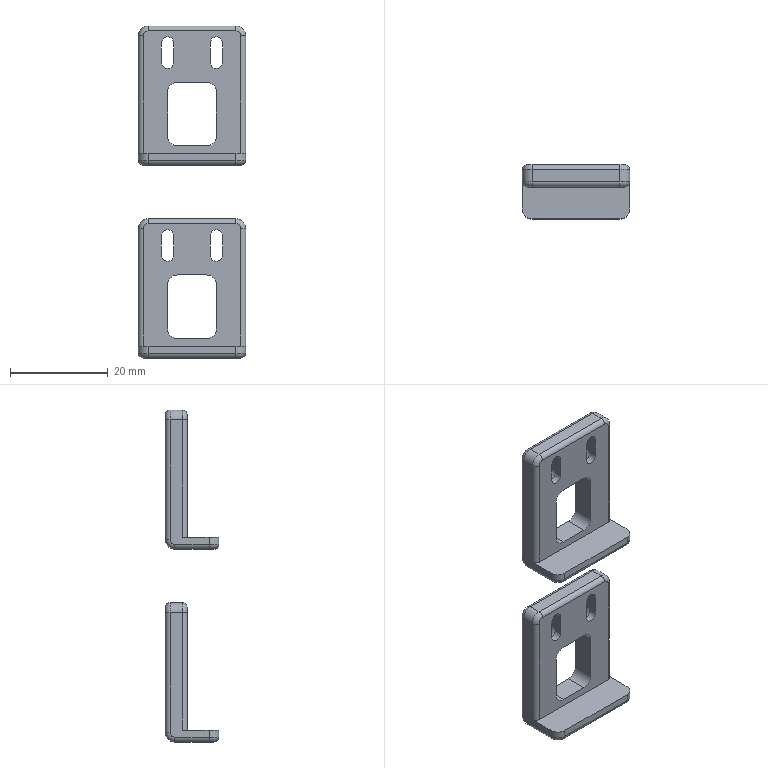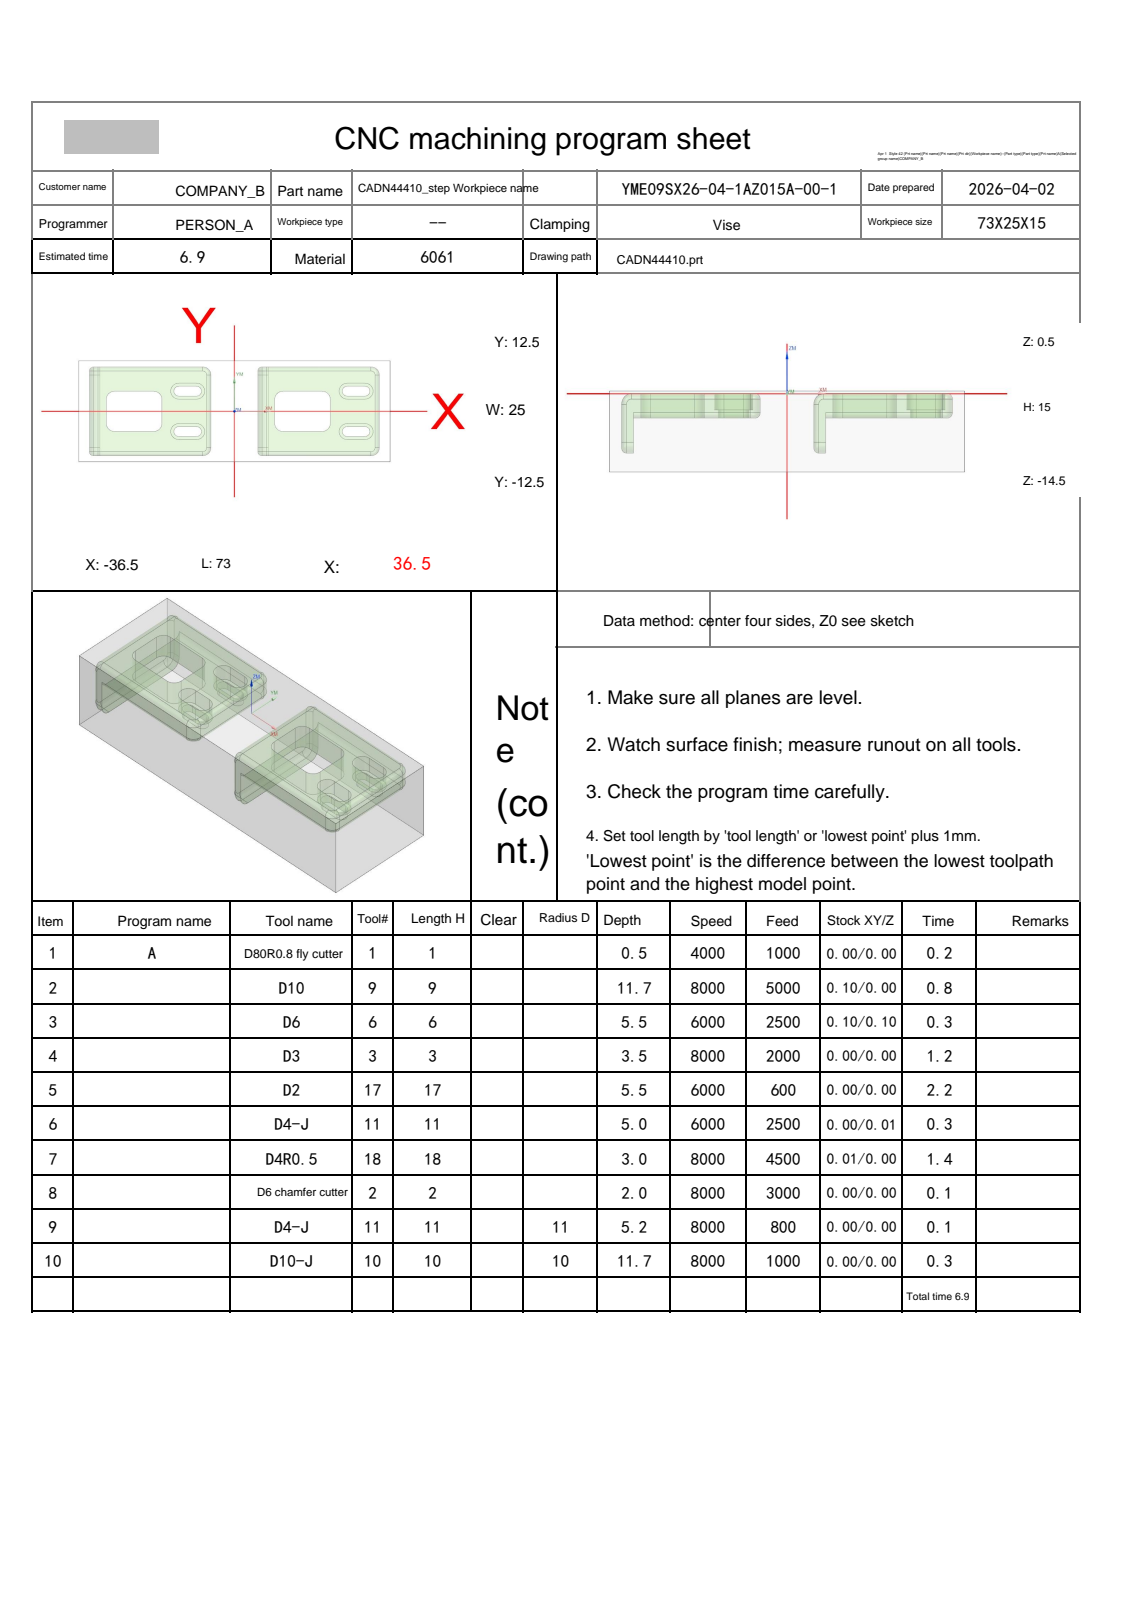NC program | NX | posted by the shop | part box 22 x 11 x 68 mm
Lines 2101 to 3074 of 7842:
N5 T17 M06
(D2  D=2. R=0. H=17 ce=0.10 di=0.10)
G00 G90 G54 X-10.955 Y-5.15 M03 S6000
G43 H17 Z20.
M08
Z-2.5
G01 X-8.955 Z-2.517 F600.
G03 X-8.805 Y-5. Z-2.52 I0.0 J.15
X-8.955 Y-4.85 Z-2.522 I-.15 J0.0
G01 X-12.955 Z-2.557
G03 X-13.105 Y-5. Z-2.559 I0.0 J-.15
X-12.955 Y-5.15 Z-2.561 I.15 J0.0
G01 X-8.955 Z-2.596
G03 X-8.805 Y-5. Z-2.598 I0.0 J.15
X-8.955 Y-4.85 Z-2.6 I-.15 J0.0
G01 X-12.955 Z-2.635
G03 X-13.105 Y-5. Z-2.637 I0.0 J-.15
X-12.955 Y-5.15 Z-2.639 I.15 J0.0
G01 X-8.955 Z-2.674
G03 X-8.805 Y-5. Z-2.676 I0.0 J.15
X-8.955 Y-4.85 Z-2.678 I-.15 J0.0
G01 X-12.955 Z-2.713
G03 X-13.105 Y-5. Z-2.715 I0.0 J-.15
X-12.955 Y-5.15 Z-2.717 I.15 J0.0
G01 X-8.955 Z-2.752
G03 X-8.805 Y-5. Z-2.754 I0.0 J.15
X-8.955 Y-4.85 Z-2.756 I-.15 J0.0
G01 X-12.955 Z-2.791
G03 X-13.105 Y-5. Z-2.793 I0.0 J-.15
X-12.955 Y-5.15 Z-2.795 I.15 J0.0
G01 X-8.955 Z-2.83
G03 X-8.805 Y-5. Z-2.832 I0.0 J.15
X-8.955 Y-4.85 Z-2.834 I-.15 J0.0
G01 X-12.955 Z-2.869
G03 X-13.105 Y-5. Z-2.871 I0.0 J-.15
X-12.955 Y-5.15 Z-2.873 I.15 J0.0
G01 X-8.955 Z-2.908
G03 X-8.805 Y-5. Z-2.91 I0.0 J.15
X-8.955 Y-4.85 Z-2.912 I-.15 J0.0
G01 X-12.955 Z-2.947
G03 X-13.105 Y-5. Z-2.949 I0.0 J-.15
X-12.955 Y-5.15 Z-2.951 I.15 J0.0
G01 X-8.955 Z-2.986
G03 X-8.805 Y-5. Z-2.988 I0.0 J.15
X-8.955 Y-4.85 Z-2.99 I-.15 J0.0
G01 X-12.955 Z-3.025
G03 X-13.105 Y-5. Z-3.027 I0.0 J-.15
X-12.955 Y-5.15 Z-3.029 I.15 J0.0
G01 X-8.955 Z-3.064
G03 X-8.805 Y-5. Z-3.066 I0.0 J.15
X-8.955 Y-4.85 Z-3.068 I-.15 J0.0
G01 X-12.955 Z-3.103
G03 X-13.105 Y-5. Z-3.105 I0.0 J-.15
X-12.955 Y-5.15 Z-3.108 I.15 J0.0
G01 X-8.955 Z-3.142
G03 X-8.805 Y-5. Z-3.145 I0.0 J.15
X-8.955 Y-4.85 Z-3.147 I-.15 J0.0
G01 X-12.955 Z-3.182
G03 X-13.105 Y-5. Z-3.184 I0.0 J-.15
X-12.955 Y-5.15 Z-3.186 I.15 J0.0
G01 X-8.955 Z-3.221
G03 X-8.805 Y-5. Z-3.223 I0.0 J.15
X-8.955 Y-4.85 Z-3.225 I-.15 J0.0
G01 X-12.955 Z-3.26
G03 X-13.105 Y-5. Z-3.262 I0.0 J-.15
X-12.955 Y-5.15 Z-3.264 I.15 J0.0
G01 X-8.955 Z-3.299
G03 X-8.805 Y-5. Z-3.301 I0.0 J.15
X-8.955 Y-4.85 Z-3.303 I-.15 J0.0
G01 X-12.955 Z-3.338
G03 X-13.105 Y-5. Z-3.34 I0.0 J-.15
X-12.955 Y-5.15 Z-3.342 I.15 J0.0
G01 X-8.955 Z-3.377
G03 X-8.805 Y-5. Z-3.379 I0.0 J.15
X-8.955 Y-4.85 Z-3.381 I-.15 J0.0
G01 X-12.955 Z-3.416
G03 X-13.105 Y-5. Z-3.418 I0.0 J-.15
X-12.955 Y-5.15 Z-3.42 I.15 J0.0
G01 X-8.955 Z-3.455
G03 X-8.805 Y-5. Z-3.457 I0.0 J.15
X-8.955 Y-4.85 Z-3.459 I-.15 J0.0
G01 X-12.955 Z-3.494
G03 X-13.105 Y-5. Z-3.496 I0.0 J-.15
X-12.955 Y-5.15 Z-3.498 I.15 J0.0
G01 X-8.955 Z-3.533
G03 X-8.805 Y-5. Z-3.535 I0.0 J.15
X-8.955 Y-4.85 Z-3.537 I-.15 J0.0
G01 X-12.955 Z-3.572
G03 X-13.105 Y-5. Z-3.574 I0.0 J-.15
X-12.955 Y-5.15 Z-3.576 I.15 J0.0
G01 X-8.955 Z-3.611
G03 X-8.805 Y-5. Z-3.613 I0.0 J.15
X-8.955 Y-4.85 Z-3.615 I-.15 J0.0
G01 X-12.955 Z-3.65
G03 X-13.105 Y-5. Z-3.652 I0.0 J-.15
X-12.955 Y-5.15 Z-3.654 I.15 J0.0
G01 X-8.955 Z-3.689
G03 X-8.805 Y-5. Z-3.691 I0.0 J.15
X-8.955 Y-4.85 Z-3.693 I-.15 J0.0
G01 X-12.955 Z-3.728
G03 X-13.105 Y-5. Z-3.73 I0.0 J-.15
X-12.955 Y-5.15 Z-3.733 I.15 J0.0
G01 X-8.955 Z-3.767
G03 X-8.805 Y-5. Z-3.77 I0.0 J.15
X-8.955 Y-4.85 Z-3.772 I-.15 J0.0
G01 X-12.955 Z-3.807
G03 X-13.105 Y-5. Z-3.809 I0.0 J-.15
X-12.955 Y-5.15 Z-3.811 I.15 J0.0
G01 X-8.955 Z-3.846
G03 X-8.805 Y-5. Z-3.848 I0.0 J.15
X-8.955 Y-4.85 Z-3.85 I-.15 J0.0
G01 X-12.955 Z-3.885
G03 X-13.105 Y-5. Z-3.887 I0.0 J-.15
X-12.955 Y-5.15 Z-3.889 I.15 J0.0
G01 X-8.955 Z-3.924
G03 X-8.805 Y-5. Z-3.926 I0.0 J.15
X-8.955 Y-4.85 Z-3.928 I-.15 J0.0
G01 X-12.955 Z-3.963
G03 X-13.105 Y-5. Z-3.965 I0.0 J-.15
X-12.955 Y-5.15 Z-3.967 I.15 J0.0
G01 X-8.955 Z-4.002
G03 X-8.805 Y-5. Z-4.004 I0.0 J.15
X-8.955 Y-4.85 Z-4.006 I-.15 J0.0
G01 X-12.955 Z-4.041
G03 X-13.105 Y-5. Z-4.043 I0.0 J-.15
X-12.955 Y-5.15 Z-4.045 I.15 J0.0
G01 X-8.955 Z-4.08
G03 X-8.805 Y-5. Z-4.082 I0.0 J.15
X-8.955 Y-4.85 Z-4.084 I-.15 J0.0
G01 X-12.955 Z-4.119
G03 X-13.105 Y-5. Z-4.121 I0.0 J-.15
X-12.955 Y-5.15 Z-4.123 I.15 J0.0
G01 X-8.955 Z-4.158
G03 X-8.805 Y-5. Z-4.16 I0.0 J.15
X-8.955 Y-4.85 Z-4.162 I-.15 J0.0
G01 X-12.955 Z-4.197
G03 X-13.105 Y-5. Z-4.199 I0.0 J-.15
X-12.955 Y-5.15 Z-4.201 I.15 J0.0
G01 X-8.955 Z-4.236
G03 X-8.805 Y-5. Z-4.238 I0.0 J.15
X-8.955 Y-4.85 Z-4.24 I-.15 J0.0
G01 X-12.955 Z-4.275
G03 X-13.105 Y-5. Z-4.277 I0.0 J-.15
X-12.955 Y-5.15 Z-4.279 I.15 J0.0
G01 X-8.955 Z-4.314
G03 X-8.805 Y-5. Z-4.316 I0.0 J.15
X-8.955 Y-4.85 Z-4.318 I-.15 J0.0
G01 X-12.955 Z-4.353
G03 X-13.105 Y-5. Z-4.355 I0.0 J-.15
X-12.955 Y-5.15 Z-4.358 I.15 J0.0
G01 X-8.955 Z-4.392
G03 X-8.805 Y-5. Z-4.395 I0.0 J.15
X-8.955 Y-4.85 Z-4.397 I-.15 J0.0
G01 X-12.955 Z-4.432
G03 X-13.105 Y-5. Z-4.434 I0.0 J-.15
X-12.955 Y-5.15 Z-4.436 I.15 J0.0
G01 X-8.955 Z-4.471
G03 X-8.805 Y-5. Z-4.473 I0.0 J.15
X-8.955 Y-4.85 Z-4.475 I-.15 J0.0
G01 X-12.955 Z-4.51
G03 X-13.105 Y-5. Z-4.512 I0.0 J-.15
X-12.955 Y-5.15 Z-4.514 I.15 J0.0
G01 X-8.955 Z-4.549
G03 X-8.805 Y-5. Z-4.551 I0.0 J.15
X-8.955 Y-4.85 Z-4.553 I-.15 J0.0
G01 X-12.955 Z-4.588
G03 X-13.105 Y-5. Z-4.59 I0.0 J-.15
X-12.955 Y-5.15 Z-4.592 I.15 J0.0
G01 X-8.955 Z-4.627
G03 X-8.805 Y-5. Z-4.629 I0.0 J.15
X-8.955 Y-4.85 Z-4.631 I-.15 J0.0
G01 X-12.955 Z-4.666
G03 X-13.105 Y-5. Z-4.668 I0.0 J-.15
X-12.955 Y-5.15 Z-4.67 I.15 J0.0
G01 X-8.955 Z-4.705
G03 X-8.805 Y-5. Z-4.707 I0.0 J.15
X-8.955 Y-4.85 Z-4.709 I-.15 J0.0
G01 X-12.955 Z-4.744
G03 X-13.105 Y-5. Z-4.746 I0.0 J-.15
X-12.955 Y-5.15 Z-4.748 I.15 J0.0
G01 X-8.955 Z-4.783
G03 X-8.805 Y-5. Z-4.785 I0.0 J.15
X-8.955 Y-4.85 Z-4.787 I-.15 J0.0
G01 X-12.955 Z-4.822
G03 X-13.105 Y-5. Z-4.824 I0.0 J-.15
X-12.955 Y-5.15 Z-4.826 I.15 J0.0
G01 X-8.955 Z-4.861
G03 X-8.805 Y-5. Z-4.863 I0.0 J.15
X-8.955 Y-4.85 Z-4.865 I-.15 J0.0
G01 X-12.955 Z-4.9
G03 X-13.105 Y-5. Z-4.902 I0.0 J-.15
X-12.955 Y-5.15 Z-4.904 I.15 J0.0
G01 X-8.955 Z-4.939
G03 X-8.805 Y-5. Z-4.941 I0.0 J.15
X-8.955 Y-4.85 Z-4.943 I-.15 J0.0
G01 X-12.955 Z-4.978
G03 X-13.105 Y-5. Z-4.98 I0.0 J-.15
X-12.955 Y-5.15 Z-4.983 I.15 J0.0
G01 X-10.955 Z-5.
X-8.955
G03 X-8.805 Y-5. I0.0 J.15
X-8.955 Y-4.85 I-.15 J0.0
G01 X-12.955
G03 X-13.105 Y-5. I0.0 J-.15
X-12.955 Y-5.15 I.15 J0.0
G01 X-10.955
X-10.455
Z-4.
G00 Z20.
X-10.955 Y5.15
Z-2.5
G01 X-12.955 Z-2.517
G03 X-13.105 Y5. Z-2.52 I0.0 J-.15
X-12.955 Y4.85 Z-2.522 I.15 J0.0
G01 X-8.955 Z-2.557
G03 X-8.805 Y5. Z-2.559 I0.0 J.15
X-8.955 Y5.15 Z-2.561 I-.15 J0.0
G01 X-12.955 Z-2.596
G03 X-13.105 Y5. Z-2.598 I0.0 J-.15
X-12.955 Y4.85 Z-2.6 I.15 J0.0
G01 X-8.955 Z-2.635
G03 X-8.805 Y5. Z-2.637 I0.0 J.15
X-8.955 Y5.15 Z-2.639 I-.15 J0.0
G01 X-12.955 Z-2.674
G03 X-13.105 Y5. Z-2.676 I0.0 J-.15
X-12.955 Y4.85 Z-2.678 I.15 J0.0
G01 X-8.955 Z-2.713
G03 X-8.805 Y5. Z-2.715 I0.0 J.15
X-8.955 Y5.15 Z-2.717 I-.15 J0.0
G01 X-12.955 Z-2.752
G03 X-13.105 Y5. Z-2.754 I0.0 J-.15
X-12.955 Y4.85 Z-2.756 I.15 J0.0
G01 X-8.955 Z-2.791
G03 X-8.805 Y5. Z-2.793 I0.0 J.15
X-8.955 Y5.15 Z-2.795 I-.15 J0.0
G01 X-12.955 Z-2.83
G03 X-13.105 Y5. Z-2.832 I0.0 J-.15
X-12.955 Y4.85 Z-2.834 I.15 J0.0
G01 X-8.955 Z-2.869
G03 X-8.805 Y5. Z-2.871 I0.0 J.15
X-8.955 Y5.15 Z-2.873 I-.15 J0.0
G01 X-12.955 Z-2.908
G03 X-13.105 Y5. Z-2.91 I0.0 J-.15
X-12.955 Y4.85 Z-2.912 I.15 J0.0
G01 X-8.955 Z-2.947
G03 X-8.805 Y5. Z-2.949 I0.0 J.15
X-8.955 Y5.15 Z-2.951 I-.15 J0.0
G01 X-12.955 Z-2.986
G03 X-13.105 Y5. Z-2.988 I0.0 J-.15
X-12.955 Y4.85 Z-2.99 I.15 J0.0
G01 X-8.955 Z-3.025
G03 X-8.805 Y5. Z-3.027 I0.0 J.15
X-8.955 Y5.15 Z-3.029 I-.15 J0.0
G01 X-12.955 Z-3.064
G03 X-13.105 Y5. Z-3.066 I0.0 J-.15
X-12.955 Y4.85 Z-3.068 I.15 J0.0
G01 X-8.955 Z-3.103
G03 X-8.805 Y5. Z-3.105 I0.0 J.15
X-8.955 Y5.15 Z-3.108 I-.15 J0.0
G01 X-12.955 Z-3.142
G03 X-13.105 Y5. Z-3.145 I0.0 J-.15
X-12.955 Y4.85 Z-3.147 I.15 J0.0
G01 X-8.955 Z-3.182
G03 X-8.805 Y5. Z-3.184 I0.0 J.15
X-8.955 Y5.15 Z-3.186 I-.15 J0.0
G01 X-12.955 Z-3.221
G03 X-13.105 Y5. Z-3.223 I0.0 J-.15
X-12.955 Y4.85 Z-3.225 I.15 J0.0
G01 X-8.955 Z-3.26
G03 X-8.805 Y5. Z-3.262 I0.0 J.15
X-8.955 Y5.15 Z-3.264 I-.15 J0.0
G01 X-12.955 Z-3.299
G03 X-13.105 Y5. Z-3.301 I0.0 J-.15
X-12.955 Y4.85 Z-3.303 I.15 J0.0
G01 X-8.955 Z-3.338
G03 X-8.805 Y5. Z-3.34 I0.0 J.15
X-8.955 Y5.15 Z-3.342 I-.15 J0.0
G01 X-12.955 Z-3.377
G03 X-13.105 Y5. Z-3.379 I0.0 J-.15
X-12.955 Y4.85 Z-3.381 I.15 J0.0
G01 X-8.955 Z-3.416
G03 X-8.805 Y5. Z-3.418 I0.0 J.15
X-8.955 Y5.15 Z-3.42 I-.15 J0.0
G01 X-12.955 Z-3.455
G03 X-13.105 Y5. Z-3.457 I0.0 J-.15
X-12.955 Y4.85 Z-3.459 I.15 J0.0
G01 X-8.955 Z-3.494
G03 X-8.805 Y5. Z-3.496 I0.0 J.15
X-8.955 Y5.15 Z-3.498 I-.15 J0.0
G01 X-12.955 Z-3.533
G03 X-13.105 Y5. Z-3.535 I0.0 J-.15
X-12.955 Y4.85 Z-3.537 I.15 J0.0
G01 X-8.955 Z-3.572
G03 X-8.805 Y5. Z-3.574 I0.0 J.15
X-8.955 Y5.15 Z-3.576 I-.15 J0.0
G01 X-12.955 Z-3.611
G03 X-13.105 Y5. Z-3.613 I0.0 J-.15
X-12.955 Y4.85 Z-3.615 I.15 J0.0
G01 X-8.955 Z-3.65
G03 X-8.805 Y5. Z-3.652 I0.0 J.15
X-8.955 Y5.15 Z-3.654 I-.15 J0.0
G01 X-12.955 Z-3.689
G03 X-13.105 Y5. Z-3.691 I0.0 J-.15
X-12.955 Y4.85 Z-3.693 I.15 J0.0
G01 X-8.955 Z-3.728
G03 X-8.805 Y5. Z-3.73 I0.0 J.15
X-8.955 Y5.15 Z-3.733 I-.15 J0.0
G01 X-12.955 Z-3.767
G03 X-13.105 Y5. Z-3.77 I0.0 J-.15
X-12.955 Y4.85 Z-3.772 I.15 J0.0
G01 X-8.955 Z-3.807
G03 X-8.805 Y5. Z-3.809 I0.0 J.15
X-8.955 Y5.15 Z-3.811 I-.15 J0.0
G01 X-12.955 Z-3.846
G03 X-13.105 Y5. Z-3.848 I0.0 J-.15
X-12.955 Y4.85 Z-3.85 I.15 J0.0
G01 X-8.955 Z-3.885
G03 X-8.805 Y5. Z-3.887 I0.0 J.15
X-8.955 Y5.15 Z-3.889 I-.15 J0.0
G01 X-12.955 Z-3.924
G03 X-13.105 Y5. Z-3.926 I0.0 J-.15
X-12.955 Y4.85 Z-3.928 I.15 J0.0
G01 X-8.955 Z-3.963
G03 X-8.805 Y5. Z-3.965 I0.0 J.15
X-8.955 Y5.15 Z-3.967 I-.15 J0.0
G01 X-12.955 Z-4.002
G03 X-13.105 Y5. Z-4.004 I0.0 J-.15
X-12.955 Y4.85 Z-4.006 I.15 J0.0
G01 X-8.955 Z-4.041
G03 X-8.805 Y5. Z-4.043 I0.0 J.15
X-8.955 Y5.15 Z-4.045 I-.15 J0.0
G01 X-12.955 Z-4.08
G03 X-13.105 Y5. Z-4.082 I0.0 J-.15
X-12.955 Y4.85 Z-4.084 I.15 J0.0
G01 X-8.955 Z-4.119
G03 X-8.805 Y5. Z-4.121 I0.0 J.15
X-8.955 Y5.15 Z-4.123 I-.15 J0.0
G01 X-12.955 Z-4.158
G03 X-13.105 Y5. Z-4.16 I0.0 J-.15
X-12.955 Y4.85 Z-4.162 I.15 J0.0
G01 X-8.955 Z-4.197
G03 X-8.805 Y5. Z-4.199 I0.0 J.15
X-8.955 Y5.15 Z-4.201 I-.15 J0.0
G01 X-12.955 Z-4.236
G03 X-13.105 Y5. Z-4.238 I0.0 J-.15
X-12.955 Y4.85 Z-4.24 I.15 J0.0
G01 X-8.955 Z-4.275
G03 X-8.805 Y5. Z-4.277 I0.0 J.15
X-8.955 Y5.15 Z-4.279 I-.15 J0.0
G01 X-12.955 Z-4.314
G03 X-13.105 Y5. Z-4.316 I0.0 J-.15
X-12.955 Y4.85 Z-4.318 I.15 J0.0
G01 X-8.955 Z-4.353
G03 X-8.805 Y5. Z-4.355 I0.0 J.15
X-8.955 Y5.15 Z-4.358 I-.15 J0.0
G01 X-12.955 Z-4.392
G03 X-13.105 Y5. Z-4.395 I0.0 J-.15
X-12.955 Y4.85 Z-4.397 I.15 J0.0
G01 X-8.955 Z-4.432
G03 X-8.805 Y5. Z-4.434 I0.0 J.15
X-8.955 Y5.15 Z-4.436 I-.15 J0.0
G01 X-12.955 Z-4.471
G03 X-13.105 Y5. Z-4.473 I0.0 J-.15
X-12.955 Y4.85 Z-4.475 I.15 J0.0
G01 X-8.955 Z-4.51
G03 X-8.805 Y5. Z-4.512 I0.0 J.15
X-8.955 Y5.15 Z-4.514 I-.15 J0.0
G01 X-12.955 Z-4.549
G03 X-13.105 Y5. Z-4.551 I0.0 J-.15
X-12.955 Y4.85 Z-4.553 I.15 J0.0
G01 X-8.955 Z-4.588
G03 X-8.805 Y5. Z-4.59 I0.0 J.15
X-8.955 Y5.15 Z-4.592 I-.15 J0.0
G01 X-12.955 Z-4.627
G03 X-13.105 Y5. Z-4.629 I0.0 J-.15
X-12.955 Y4.85 Z-4.631 I.15 J0.0
G01 X-8.955 Z-4.666
G03 X-8.805 Y5. Z-4.668 I0.0 J.15
X-8.955 Y5.15 Z-4.67 I-.15 J0.0
G01 X-12.955 Z-4.705
G03 X-13.105 Y5. Z-4.707 I0.0 J-.15
X-12.955 Y4.85 Z-4.709 I.15 J0.0
G01 X-8.955 Z-4.744
G03 X-8.805 Y5. Z-4.746 I0.0 J.15
X-8.955 Y5.15 Z-4.748 I-.15 J0.0
G01 X-12.955 Z-4.783
G03 X-13.105 Y5. Z-4.785 I0.0 J-.15
X-12.955 Y4.85 Z-4.787 I.15 J0.0
G01 X-8.955 Z-4.822
G03 X-8.805 Y5. Z-4.824 I0.0 J.15
X-8.955 Y5.15 Z-4.826 I-.15 J0.0
G01 X-12.955 Z-4.861
G03 X-13.105 Y5. Z-4.863 I0.0 J-.15
X-12.955 Y4.85 Z-4.865 I.15 J0.0
G01 X-8.955 Z-4.9
G03 X-8.805 Y5. Z-4.902 I0.0 J.15
X-8.955 Y5.15 Z-4.904 I-.15 J0.0
G01 X-12.955 Z-4.939
G03 X-13.105 Y5. Z-4.941 I0.0 J-.15
X-12.955 Y4.85 Z-4.943 I.15 J0.0
G01 X-8.955 Z-4.978
G03 X-8.805 Y5. Z-4.98 I0.0 J.15
X-8.955 Y5.15 Z-4.983 I-.15 J0.0
G01 X-10.955 Z-5.
X-12.955
G03 X-13.105 Y5. I0.0 J-.15
X-12.955 Y4.85 I.15 J0.0
G01 X-8.955
G03 X-8.805 Y5. I0.0 J.15
X-8.955 Y5.15 I-.15 J0.0
G01 X-10.955
X-11.455
Z-4.
G00 Z20.
X28.545
Z-2.5
G01 X26.545 Z-2.517
G03 X26.395 Y5. Z-2.52 I0.0 J-.15
X26.545 Y4.85 Z-2.522 I.15 J0.0
G01 X30.545 Z-2.557
G03 X30.695 Y5. Z-2.559 I0.0 J.15
X30.545 Y5.15 Z-2.561 I-.15 J0.0
G01 X26.545 Z-2.596
G03 X26.395 Y5. Z-2.598 I0.0 J-.15
X26.545 Y4.85 Z-2.6 I.15 J0.0
G01 X30.545 Z-2.635
G03 X30.695 Y5. Z-2.637 I0.0 J.15
X30.545 Y5.15 Z-2.639 I-.15 J0.0
G01 X26.545 Z-2.674
G03 X26.395 Y5. Z-2.676 I0.0 J-.15
X26.545 Y4.85 Z-2.678 I.15 J0.0
G01 X30.545 Z-2.713
G03 X30.695 Y5. Z-2.715 I0.0 J.15
X30.545 Y5.15 Z-2.717 I-.15 J0.0
G01 X26.545 Z-2.752
G03 X26.395 Y5. Z-2.754 I0.0 J-.15
X26.545 Y4.85 Z-2.756 I.15 J0.0
G01 X30.545 Z-2.791
G03 X30.695 Y5. Z-2.793 I0.0 J.15
X30.545 Y5.15 Z-2.795 I-.15 J0.0
G01 X26.545 Z-2.83
G03 X26.395 Y5. Z-2.832 I0.0 J-.15
X26.545 Y4.85 Z-2.834 I.15 J0.0
G01 X30.545 Z-2.869
G03 X30.695 Y5. Z-2.871 I0.0 J.15
X30.545 Y5.15 Z-2.873 I-.15 J0.0
G01 X26.545 Z-2.908
G03 X26.395 Y5. Z-2.91 I0.0 J-.15
X26.545 Y4.85 Z-2.912 I.15 J0.0
G01 X30.545 Z-2.947
G03 X30.695 Y5. Z-2.949 I0.0 J.15
X30.545 Y5.15 Z-2.951 I-.15 J0.0
G01 X26.545 Z-2.986
G03 X26.395 Y5. Z-2.988 I0.0 J-.15
X26.545 Y4.85 Z-2.99 I.15 J0.0
G01 X30.545 Z-3.025
G03 X30.695 Y5. Z-3.027 I0.0 J.15
X30.545 Y5.15 Z-3.029 I-.15 J0.0
G01 X26.545 Z-3.064
G03 X26.395 Y5. Z-3.066 I0.0 J-.15
X26.545 Y4.85 Z-3.068 I.15 J0.0
G01 X30.545 Z-3.103
G03 X30.695 Y5. Z-3.105 I0.0 J.15
X30.545 Y5.15 Z-3.108 I-.15 J0.0
G01 X26.545 Z-3.142
G03 X26.395 Y5. Z-3.145 I0.0 J-.15
X26.545 Y4.85 Z-3.147 I.15 J0.0
G01 X30.545 Z-3.182
G03 X30.695 Y5. Z-3.184 I0.0 J.15
X30.545 Y5.15 Z-3.186 I-.15 J0.0
G01 X26.545 Z-3.221
G03 X26.395 Y5. Z-3.223 I0.0 J-.15
X26.545 Y4.85 Z-3.225 I.15 J0.0
G01 X30.545 Z-3.26
G03 X30.695 Y5. Z-3.262 I0.0 J.15
X30.545 Y5.15 Z-3.264 I-.15 J0.0
G01 X26.545 Z-3.299
G03 X26.395 Y5. Z-3.301 I0.0 J-.15
X26.545 Y4.85 Z-3.303 I.15 J0.0
G01 X30.545 Z-3.338
G03 X30.695 Y5. Z-3.34 I0.0 J.15
X30.545 Y5.15 Z-3.342 I-.15 J0.0
G01 X26.545 Z-3.377
G03 X26.395 Y5. Z-3.379 I0.0 J-.15
X26.545 Y4.85 Z-3.381 I.15 J0.0
G01 X30.545 Z-3.416
G03 X30.695 Y5. Z-3.418 I0.0 J.15
X30.545 Y5.15 Z-3.42 I-.15 J0.0
G01 X26.545 Z-3.455
G03 X26.395 Y5. Z-3.457 I0.0 J-.15
X26.545 Y4.85 Z-3.459 I.15 J0.0
G01 X30.545 Z-3.494
G03 X30.695 Y5. Z-3.496 I0.0 J.15
X30.545 Y5.15 Z-3.498 I-.15 J0.0
G01 X26.545 Z-3.533
G03 X26.395 Y5. Z-3.535 I0.0 J-.15
X26.545 Y4.85 Z-3.537 I.15 J0.0
G01 X30.545 Z-3.572
G03 X30.695 Y5. Z-3.574 I0.0 J.15
X30.545 Y5.15 Z-3.576 I-.15 J0.0
G01 X26.545 Z-3.611
G03 X26.395 Y5. Z-3.613 I0.0 J-.15
X26.545 Y4.85 Z-3.615 I.15 J0.0
G01 X30.545 Z-3.65
G03 X30.695 Y5. Z-3.652 I0.0 J.15
X30.545 Y5.15 Z-3.654 I-.15 J0.0
G01 X26.545 Z-3.689
G03 X26.395 Y5. Z-3.691 I0.0 J-.15
X26.545 Y4.85 Z-3.693 I.15 J0.0
G01 X30.545 Z-3.728
G03 X30.695 Y5. Z-3.73 I0.0 J.15
X30.545 Y5.15 Z-3.733 I-.15 J0.0
G01 X26.545 Z-3.767
G03 X26.395 Y5. Z-3.77 I0.0 J-.15
X26.545 Y4.85 Z-3.772 I.15 J0.0
G01 X30.545 Z-3.807
G03 X30.695 Y5. Z-3.809 I0.0 J.15
X30.545 Y5.15 Z-3.811 I-.15 J0.0
G01 X26.545 Z-3.846
G03 X26.395 Y5. Z-3.848 I0.0 J-.15
X26.545 Y4.85 Z-3.85 I.15 J0.0
G01 X30.545 Z-3.885
G03 X30.695 Y5. Z-3.887 I0.0 J.15
X30.545 Y5.15 Z-3.889 I-.15 J0.0
G01 X26.545 Z-3.924
G03 X26.395 Y5. Z-3.926 I0.0 J-.15
X26.545 Y4.85 Z-3.928 I.15 J0.0
G01 X30.545 Z-3.963
G03 X30.695 Y5. Z-3.965 I0.0 J.15
X30.545 Y5.15 Z-3.967 I-.15 J0.0
G01 X26.545 Z-4.002
G03 X26.395 Y5. Z-4.004 I0.0 J-.15
X26.545 Y4.85 Z-4.006 I.15 J0.0
G01 X30.545 Z-4.041
G03 X30.695 Y5. Z-4.043 I0.0 J.15
X30.545 Y5.15 Z-4.045 I-.15 J0.0
G01 X26.545 Z-4.08
G03 X26.395 Y5. Z-4.082 I0.0 J-.15
X26.545 Y4.85 Z-4.084 I.15 J0.0
G01 X30.545 Z-4.119
G03 X30.695 Y5. Z-4.121 I0.0 J.15
X30.545 Y5.15 Z-4.123 I-.15 J0.0
G01 X26.545 Z-4.158
G03 X26.395 Y5. Z-4.16 I0.0 J-.15
X26.545 Y4.85 Z-4.162 I.15 J0.0
G01 X30.545 Z-4.197
G03 X30.695 Y5. Z-4.199 I0.0 J.15
X30.545 Y5.15 Z-4.201 I-.15 J0.0
G01 X26.545 Z-4.236
G03 X26.395 Y5. Z-4.238 I0.0 J-.15
X26.545 Y4.85 Z-4.24 I.15 J0.0
G01 X30.545 Z-4.275
G03 X30.695 Y5. Z-4.277 I0.0 J.15
X30.545 Y5.15 Z-4.279 I-.15 J0.0
G01 X26.545 Z-4.314
G03 X26.395 Y5. Z-4.316 I0.0 J-.15
X26.545 Y4.85 Z-4.318 I.15 J0.0
G01 X30.545 Z-4.353
G03 X30.695 Y5. Z-4.355 I0.0 J.15
X30.545 Y5.15 Z-4.358 I-.15 J0.0
G01 X26.545 Z-4.392
G03 X26.395 Y5. Z-4.395 I0.0 J-.15
X26.545 Y4.85 Z-4.397 I.15 J0.0
G01 X30.545 Z-4.432
G03 X30.695 Y5. Z-4.434 I0.0 J.15
X30.545 Y5.15 Z-4.436 I-.15 J0.0
G01 X26.545 Z-4.471
G03 X26.395 Y5. Z-4.473 I0.0 J-.15
X26.545 Y4.85 Z-4.475 I.15 J0.0
G01 X30.545 Z-4.51
G03 X30.695 Y5. Z-4.512 I0.0 J.15
X30.545 Y5.15 Z-4.514 I-.15 J0.0
G01 X26.545 Z-4.549
G03 X26.395 Y5. Z-4.551 I0.0 J-.15
X26.545 Y4.85 Z-4.553 I.15 J0.0
G01 X30.545 Z-4.588
G03 X30.695 Y5. Z-4.59 I0.0 J.15
X30.545 Y5.15 Z-4.592 I-.15 J0.0
G01 X26.545 Z-4.627
G03 X26.395 Y5. Z-4.629 I0.0 J-.15
X26.545 Y4.85 Z-4.631 I.15 J0.0
G01 X30.545 Z-4.666
G03 X30.695 Y5. Z-4.668 I0.0 J.15
X30.545 Y5.15 Z-4.67 I-.15 J0.0
G01 X26.545 Z-4.705
G03 X26.395 Y5. Z-4.707 I0.0 J-.15
X26.545 Y4.85 Z-4.709 I.15 J0.0
G01 X30.545 Z-4.744
G03 X30.695 Y5. Z-4.746 I0.0 J.15
X30.545 Y5.15 Z-4.748 I-.15 J0.0
G01 X26.545 Z-4.783
G03 X26.395 Y5. Z-4.785 I0.0 J-.15
X26.545 Y4.85 Z-4.787 I.15 J0.0
G01 X30.545 Z-4.822
G03 X30.695 Y5. Z-4.824 I0.0 J.15
X30.545 Y5.15 Z-4.826 I-.15 J0.0
G01 X26.545 Z-4.861
G03 X26.395 Y5. Z-4.863 I0.0 J-.15
X26.545 Y4.85 Z-4.865 I.15 J0.0
G01 X30.545 Z-4.9
G03 X30.695 Y5. Z-4.902 I0.0 J.15
X30.545 Y5.15 Z-4.904 I-.15 J0.0
G01 X26.545 Z-4.939
G03 X26.395 Y5. Z-4.941 I0.0 J-.15
X26.545 Y4.85 Z-4.943 I.15 J0.0
G01 X30.545 Z-4.978
G03 X30.695 Y5. Z-4.98 I0.0 J.15
X30.545 Y5.15 Z-4.983 I-.15 J0.0
G01 X28.545 Z-5.
X26.545
G03 X26.395 Y5. I0.0 J-.15
X26.545 Y4.85 I.15 J0.0
G01 X30.545
G03 X30.695 Y5. I0.0 J.15
X30.545 Y5.15 I-.15 J0.0
G01 X28.545
X28.045
Z-4.
G00 Z20.
X28.545 Y-5.15
Z-2.5
G01 X30.545 Z-2.517
G03 X30.695 Y-5. Z-2.52 I0.0 J.15
X30.545 Y-4.85 Z-2.522 I-.15 J0.0
G01 X26.545 Z-2.557
G03 X26.395 Y-5. Z-2.559 I0.0 J-.15
X26.545 Y-5.15 Z-2.561 I.15 J0.0
G01 X30.545 Z-2.596
G03 X30.695 Y-5. Z-2.598 I0.0 J.15
X30.545 Y-4.85 Z-2.6 I-.15 J0.0
G01 X26.545 Z-2.635
G03 X26.395 Y-5. Z-2.637 I0.0 J-.15
X26.545 Y-5.15 Z-2.639 I.15 J0.0
G01 X30.545 Z-2.674
G03 X30.695 Y-5. Z-2.676 I0.0 J.15
X30.545 Y-4.85 Z-2.678 I-.15 J0.0
G01 X26.545 Z-2.713
G03 X26.395 Y-5. Z-2.715 I0.0 J-.15
X26.545 Y-5.15 Z-2.717 I.15 J0.0
G01 X30.545 Z-2.752
G03 X30.695 Y-5. Z-2.754 I0.0 J.15
X30.545 Y-4.85 Z-2.756 I-.15 J0.0
G01 X26.545 Z-2.791
G03 X26.395 Y-5. Z-2.793 I0.0 J-.15
X26.545 Y-5.15 Z-2.795 I.15 J0.0
G01 X30.545 Z-2.83
G03 X30.695 Y-5. Z-2.832 I0.0 J.15
X30.545 Y-4.85 Z-2.834 I-.15 J0.0
G01 X26.545 Z-2.869
G03 X26.395 Y-5. Z-2.871 I0.0 J-.15
X26.545 Y-5.15 Z-2.873 I.15 J0.0
G01 X30.545 Z-2.908
G03 X30.695 Y-5. Z-2.91 I0.0 J.15
X30.545 Y-4.85 Z-2.912 I-.15 J0.0
G01 X26.545 Z-2.947
G03 X26.395 Y-5. Z-2.949 I0.0 J-.15
X26.545 Y-5.15 Z-2.951 I.15 J0.0
G01 X30.545 Z-2.986
G03 X30.695 Y-5. Z-2.988 I0.0 J.15
X30.545 Y-4.85 Z-2.99 I-.15 J0.0
G01 X26.545 Z-3.025
G03 X26.395 Y-5. Z-3.027 I0.0 J-.15
X26.545 Y-5.15 Z-3.029 I.15 J0.0
G01 X30.545 Z-3.064
G03 X30.695 Y-5. Z-3.066 I0.0 J.15
X30.545 Y-4.85 Z-3.068 I-.15 J0.0
G01 X26.545 Z-3.103
G03 X26.395 Y-5. Z-3.105 I0.0 J-.15
X26.545 Y-5.15 Z-3.108 I.15 J0.0
G01 X30.545 Z-3.142
G03 X30.695 Y-5. Z-3.145 I0.0 J.15
X30.545 Y-4.85 Z-3.147 I-.15 J0.0
G01 X26.545 Z-3.182
G03 X26.395 Y-5. Z-3.184 I0.0 J-.15
X26.545 Y-5.15 Z-3.186 I.15 J0.0
G01 X30.545 Z-3.221
G03 X30.695 Y-5. Z-3.223 I0.0 J.15
X30.545 Y-4.85 Z-3.225 I-.15 J0.0
G01 X26.545 Z-3.26
G03 X26.395 Y-5. Z-3.262 I0.0 J-.15
X26.545 Y-5.15 Z-3.264 I.15 J0.0
G01 X30.545 Z-3.299
G03 X30.695 Y-5. Z-3.301 I0.0 J.15
X30.545 Y-4.85 Z-3.303 I-.15 J0.0
G01 X26.545 Z-3.338
G03 X26.395 Y-5. Z-3.34 I0.0 J-.15
X26.545 Y-5.15 Z-3.342 I.15 J0.0
G01 X30.545 Z-3.377
G03 X30.695 Y-5. Z-3.379 I0.0 J.15
X30.545 Y-4.85 Z-3.381 I-.15 J0.0
G01 X26.545 Z-3.416
G03 X26.395 Y-5. Z-3.418 I0.0 J-.15
X26.545 Y-5.15 Z-3.42 I.15 J0.0
G01 X30.545 Z-3.455
G03 X30.695 Y-5. Z-3.457 I0.0 J.15
X30.545 Y-4.85 Z-3.459 I-.15 J0.0
G01 X26.545 Z-3.494
G03 X26.395 Y-5. Z-3.496 I0.0 J-.15
X26.545 Y-5.15 Z-3.498 I.15 J0.0
G01 X30.545 Z-3.533
G03 X30.695 Y-5. Z-3.535 I0.0 J.15
X30.545 Y-4.85 Z-3.537 I-.15 J0.0
G01 X26.545 Z-3.572
G03 X26.395 Y-5. Z-3.574 I0.0 J-.15
X26.545 Y-5.15 Z-3.576 I.15 J0.0
G01 X30.545 Z-3.611
G03 X30.695 Y-5. Z-3.613 I0.0 J.15
X30.545 Y-4.85 Z-3.615 I-.15 J0.0
G01 X26.545 Z-3.65
G03 X26.395 Y-5. Z-3.652 I0.0 J-.15
X26.545 Y-5.15 Z-3.654 I.15 J0.0
G01 X30.545 Z-3.689
G03 X30.695 Y-5. Z-3.691 I0.0 J.15
X30.545 Y-4.85 Z-3.693 I-.15 J0.0
G01 X26.545 Z-3.728
G03 X26.395 Y-5. Z-3.73 I0.0 J-.15
X26.545 Y-5.15 Z-3.733 I.15 J0.0
G01 X30.545 Z-3.767
G03 X30.695 Y-5. Z-3.77 I0.0 J.15
X30.545 Y-4.85 Z-3.772 I-.15 J0.0
G01 X26.545 Z-3.807
G03 X26.395 Y-5. Z-3.809 I0.0 J-.15
X26.545 Y-5.15 Z-3.811 I.15 J0.0
G01 X30.545 Z-3.846
G03 X30.695 Y-5. Z-3.848 I0.0 J.15
X30.545 Y-4.85 Z-3.85 I-.15 J0.0
G01 X26.545 Z-3.885
G03 X26.395 Y-5. Z-3.887 I0.0 J-.15
X26.545 Y-5.15 Z-3.889 I.15 J0.0
G01 X30.545 Z-3.924
G03 X30.695 Y-5. Z-3.926 I0.0 J.15
X30.545 Y-4.85 Z-3.928 I-.15 J0.0
G01 X26.545 Z-3.963
G03 X26.395 Y-5. Z-3.965 I0.0 J-.15
X26.545 Y-5.15 Z-3.967 I.15 J0.0
G01 X30.545 Z-4.002
G03 X30.695 Y-5. Z-4.004 I0.0 J.15
X30.545 Y-4.85 Z-4.006 I-.15 J0.0
G01 X26.545 Z-4.041
G03 X26.395 Y-5. Z-4.043 I0.0 J-.15
X26.545 Y-5.15 Z-4.045 I.15 J0.0
G01 X30.545 Z-4.08
G03 X30.695 Y-5. Z-4.082 I0.0 J.15
X30.545 Y-4.85 Z-4.084 I-.15 J0.0
G01 X26.545 Z-4.119
G03 X26.395 Y-5. Z-4.121 I0.0 J-.15
X26.545 Y-5.15 Z-4.123 I.15 J0.0
G01 X30.545 Z-4.158
G03 X30.695 Y-5. Z-4.16 I0.0 J.15
X30.545 Y-4.85 Z-4.162 I-.15 J0.0
G01 X26.545 Z-4.197
G03 X26.395 Y-5. Z-4.199 I0.0 J-.15
X26.545 Y-5.15 Z-4.201 I.15 J0.0
G01 X30.545 Z-4.236
G03 X30.695 Y-5. Z-4.238 I0.0 J.15
X30.545 Y-4.85 Z-4.24 I-.15 J0.0
G01 X26.545 Z-4.275
G03 X26.395 Y-5. Z-4.277 I0.0 J-.15
X26.545 Y-5.15 Z-4.279 I.15 J0.0
G01 X30.545 Z-4.314
G03 X30.695 Y-5. Z-4.316 I0.0 J.15
X30.545 Y-4.85 Z-4.318 I-.15 J0.0
G01 X26.545 Z-4.353
G03 X26.395 Y-5. Z-4.355 I0.0 J-.15
X26.545 Y-5.15 Z-4.358 I.15 J0.0
G01 X30.545 Z-4.392
G03 X30.695 Y-5. Z-4.395 I0.0 J.15
X30.545 Y-4.85 Z-4.397 I-.15 J0.0
G01 X26.545 Z-4.432
G03 X26.395 Y-5. Z-4.434 I0.0 J-.15
X26.545 Y-5.15 Z-4.436 I.15 J0.0
G01 X30.545 Z-4.471
G03 X30.695 Y-5. Z-4.473 I0.0 J.15
X30.545 Y-4.85 Z-4.475 I-.15 J0.0
G01 X26.545 Z-4.51
G03 X26.395 Y-5. Z-4.512 I0.0 J-.15
X26.545 Y-5.15 Z-4.514 I.15 J0.0
G01 X30.545 Z-4.549
G03 X30.695 Y-5. Z-4.551 I0.0 J.15
X30.545 Y-4.85 Z-4.553 I-.15 J0.0
G01 X26.545 Z-4.588
G03 X26.395 Y-5. Z-4.59 I0.0 J-.15
X26.545 Y-5.15 Z-4.592 I.15 J0.0
G01 X30.545 Z-4.627
G03 X30.695 Y-5. Z-4.629 I0.0 J.15
X30.545 Y-4.85 Z-4.631 I-.15 J0.0
G01 X26.545 Z-4.666
G03 X26.395 Y-5. Z-4.668 I0.0 J-.15
X26.545 Y-5.15 Z-4.67 I.15 J0.0
G01 X30.545 Z-4.705
G03 X30.695 Y-5. Z-4.707 I0.0 J.15
X30.545 Y-4.85 Z-4.709 I-.15 J0.0
G01 X26.545 Z-4.744
G03 X26.395 Y-5. Z-4.746 I0.0 J-.15
X26.545 Y-5.15 Z-4.748 I.15 J0.0
G01 X30.545 Z-4.783
G03 X30.695 Y-5. Z-4.785 I0.0 J.15
X30.545 Y-4.85 Z-4.787 I-.15 J0.0
G01 X26.545 Z-4.822
G03 X26.395 Y-5. Z-4.824 I0.0 J-.15
X26.545 Y-5.15 Z-4.826 I.15 J0.0
G01 X30.545 Z-4.861
G03 X30.695 Y-5. Z-4.863 I0.0 J.15
X30.545 Y-4.85 Z-4.865 I-.15 J0.0
G01 X26.545 Z-4.9
G03 X26.395 Y-5. Z-4.902 I0.0 J-.15
X26.545 Y-5.15 Z-4.904 I.15 J0.0
G01 X30.545 Z-4.939
G03 X30.695 Y-5. Z-4.941 I0.0 J.15
X30.545 Y-4.85 Z-4.943 I-.15 J0.0
G01 X26.545 Z-4.978
G03 X26.395 Y-5. Z-4.98 I0.0 J-.15
X26.545 Y-5.15 Z-4.983 I.15 J0.0
G01 X28.545 Z-5.
X30.545
G03 X30.695 Y-5. I0.0 J.15
X30.545 Y-4.85 I-.15 J0.0
G01 X26.545
G03 X26.395 Y-5. I0.0 J-.15
X26.545 Y-5.15 I.15 J0.0
G01 X28.545
X29.045
Z-4.
G00 Z20.
G00 G90 X-11.155 Y-5. M03 S6000
Z20.
Z-3.5
G01 Z-4. F500.
G41 D17
Y-5.05
G03 X-10.955 Y-5.25 I.2 J0.0
G01 X-8.955
G03 X-8.705 Y-5. I0.0 J.25
X-8.955 Y-4.75 I-.25 J0.0
G01 X-12.955
G03 X-13.205 Y-5. I0.0 J-.25
X-12.955 Y-5.25 I.25 J0.0
G01 X-10.955
X-10.455
G03 X-10.255 Y-5.05 I0.0 J.2
G01 G40 Y-5.
Z-3.5
G00 Z-2.
X-11.155
Z-4.5
G01 Z-5.
G41 D17
Y-5.05
G03 X-10.955 Y-5.25 I.2 J0.0
G01 X-8.955
G03 X-8.705 Y-5. I0.0 J.25
X-8.955 Y-4.75 I-.25 J0.0
G01 X-12.955
G03 X-13.205 Y-5. I0.0 J-.25
X-12.955 Y-5.25 I.25 J0.0
G01 X-10.955
X-10.455
G03 X-10.255 Y-5.05 I0.0 J.2
G01 G40 Y-5.
Z-4.5
G00 Z20.
X-10.755 Y5.
Z-3.5
G01 Z-4.
G41 D17
Y5.05
G03 X-10.955 Y5.25 I-.2 J0.0
G01 X-12.955
G03 X-13.205 Y5. I0.0 J-.25
X-12.955 Y4.75 I.25 J0.0
G01 X-8.955
G03 X-8.705 Y5. I0.0 J.25
X-8.955 Y5.25 I-.25 J0.0
G01 X-10.955
X-11.455
G03 X-11.655 Y5.05 I0.0 J-.2
G01 G40 Y5.
Z-3.5
G00 Z-2.
X-10.755
Z-4.5
G01 Z-5.
G41 D17
Y5.05
G03 X-10.955 Y5.25 I-.2 J0.0
G01 X-12.955
G03 X-13.205 Y5. I0.0 J-.25
X-12.955 Y4.75 I.25 J0.0
G01 X-8.955
G03 X-8.705 Y5. I0.0 J.25
X-8.955 Y5.25 I-.25 J0.0
G01 X-10.955
X-11.455
G03 X-11.655 Y5.05 I0.0 J-.2
G01 G40 Y5.
Z-4.5
G00 Z20.
X28.745
Z-3.5
G01 Z-4.
G41 D17
Y5.05
G03 X28.545 Y5.25 I-.2 J0.0
G01 X26.545
G03 X26.295 Y5. I0.0 J-.25
X26.545 Y4.75 I.25 J0.0
G01 X30.545
G03 X30.795 Y5. I0.0 J.25
X30.545 Y5.25 I-.25 J0.0
G01 X28.545
X28.045
G03 X27.845 Y5.05 I0.0 J-.2
G01 G40 Y5.
Z-3.5
G00 Z-2.
X28.745
Z-4.5
G01 Z-5.
G41 D17
Y5.05
G03 X28.545 Y5.25 I-.2 J0.0
G01 X26.545
G03 X26.295 Y5. I0.0 J-.25
X26.545 Y4.75 I.25 J0.0
G01 X30.545
G03 X30.795 Y5. I0.0 J.25
X30.545 Y5.25 I-.25 J0.0
G01 X28.545
X28.045
G03 X27.845 Y5.05 I0.0 J-.2
G01 G40 Y5.
Z-4.5
G00 Z20.
X28.345 Y-5.
Z-3.5
G01 Z-4.
G41 D17
Y-5.05
G03 X28.545 Y-5.25 I.2 J0.0
G01 X30.545
G03 X30.795 Y-5. I0.0 J.25
X30.545 Y-4.75 I-.25 J0.0
G01 X26.545
G03 X26.295 Y-5. I0.0 J-.25
X26.545 Y-5.25 I.25 J0.0
G01 X28.545
X29.045
G03 X29.245 Y-5.05 I0.0 J.2
G01 G40 Y-5.
Z-3.5
G00 Z-2.
X28.345
Z-4.5
G01 Z-5.
G41 D17
Y-5.05
G03 X28.545 Y-5.25 I.2 J0.0
G01 X30.545
G03 X30.795 Y-5. I0.0 J.25
X30.545 Y-4.75 I-.25 J0.0
G01 X26.545
G03 X26.295 Y-5. I0.0 J-.25
X26.545 Y-5.25 I.25 J0.0
G01 X28.545
X29.045
G03 X29.245 Y-5.05 I0.0 J.2
G01 G40 Y-5.
Z-4.5
G00 Z20.
G91 G28 Z0.0
M05
M09
G91 G28 Z0.0
M01